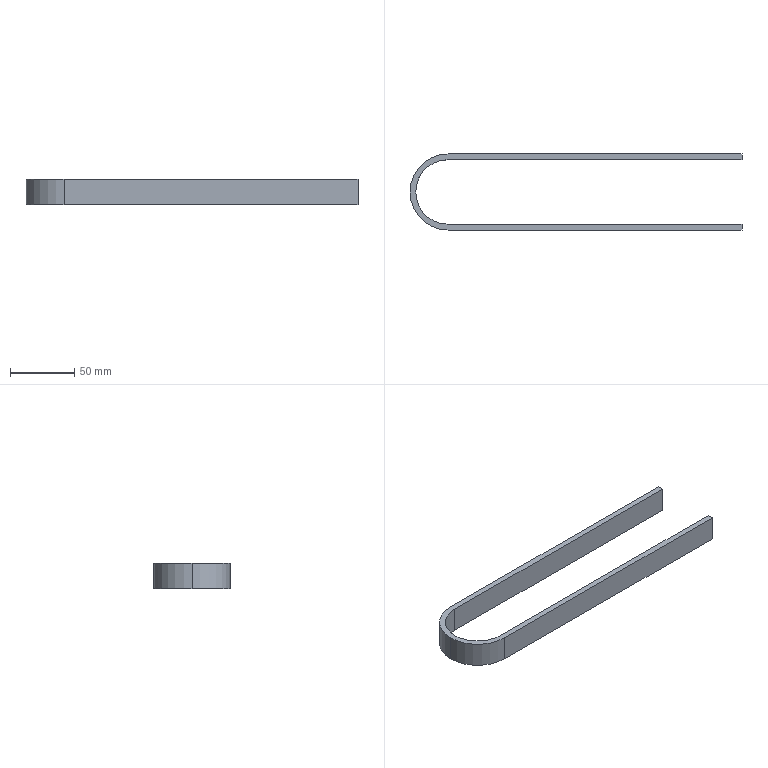Part | STEP file | Guide wheel mechanism revised.sldasm-Part-58 | 1 solid | 12 faces | box 257.5 x 59 x 20 mm | volume 48745 mm3 | plane 8 | cylinder 4 | commonest cylinder face diameters 50 x2 59 x2
STEP:
#1=CARTESIAN_POINT('',(0.,25.,10.));
#2=VERTEX_POINT('',#1);
#3=CARTESIAN_POINT('',(-25.,0.,10.));
#4=VERTEX_POINT('',#3);
#5=CARTESIAN_POINT('',(0.,0.,10.));
#6=DIRECTION('',(0.,0.,1.));
#7=DIRECTION('',(1.,0.,0.));
#8=AXIS2_PLACEMENT_3D('',#5,#6,#7);
#9=CIRCLE('',#8,25.);
#10=EDGE_CURVE('',#2,#4,#9,.T.);
#11=ORIENTED_EDGE('',*,*,#10,.T.);
#12=CARTESIAN_POINT('',(-25.,0.,-10.));
#13=VERTEX_POINT('',#12);
#14=CARTESIAN_POINT('',(-25.,0.,10.));
#15=DIRECTION('',(0.,0.,-1.));
#16=VECTOR('',#15,1000.);
#17=LINE('',#14,#16);
#18=EDGE_CURVE('',#4,#13,#17,.T.);
#19=ORIENTED_EDGE('',*,*,#18,.T.);
#20=CARTESIAN_POINT('',(0.,25.,-10.));
#21=VERTEX_POINT('',#20);
#22=CARTESIAN_POINT('',(0.,0.,-10.));
#23=DIRECTION('',(0.,0.,1.));
#24=DIRECTION('',(1.,0.,0.));
#25=AXIS2_PLACEMENT_3D('',#22,#23,#24);
#26=CIRCLE('',#25,25.);
#27=EDGE_CURVE('',#21,#13,#26,.T.);
#28=ORIENTED_EDGE('',*,*,#27,.F.);
#29=CARTESIAN_POINT('',(0.,25.,10.));
#30=DIRECTION('',(0.,0.,-1.));
#31=VECTOR('',#30,1000.);
#32=LINE('',#29,#31);
#33=EDGE_CURVE('',#2,#21,#32,.T.);
#34=ORIENTED_EDGE('',*,*,#33,.F.);
#35=EDGE_LOOP('',(#11,#19,#28,#34));
#36=FACE_OUTER_BOUND('',#35,.T.);
#37=CARTESIAN_POINT('',(0.,0.,10.));
#38=DIRECTION('',(0.,0.,-1.));
#39=DIRECTION('',(-1.,0.,0.));
#40=AXIS2_PLACEMENT_3D('',#37,#38,#39);
#41=CYLINDRICAL_SURFACE('',#40,25.);
#42=ADVANCED_FACE('',(#36),#41,.F.);
#43=CARTESIAN_POINT('',(-29.5,0.,10.));
#44=VERTEX_POINT('',#43);
#45=CARTESIAN_POINT('',(0.,-29.5,10.));
#46=VERTEX_POINT('',#45);
#47=CARTESIAN_POINT('',(0.,0.,10.));
#48=DIRECTION('',(0.,0.,1.));
#49=DIRECTION('',(1.,0.,0.));
#50=AXIS2_PLACEMENT_3D('',#47,#48,#49);
#51=CIRCLE('',#50,29.5);
#52=EDGE_CURVE('',#44,#46,#51,.T.);
#53=ORIENTED_EDGE('',*,*,#52,.F.);
#54=CARTESIAN_POINT('',(-29.5,0.,-10.));
#55=VERTEX_POINT('',#54);
#56=CARTESIAN_POINT('',(-29.5,0.,10.));
#57=DIRECTION('',(0.,0.,-1.));
#58=VECTOR('',#57,1000.);
#59=LINE('',#56,#58);
#60=EDGE_CURVE('',#44,#55,#59,.T.);
#61=ORIENTED_EDGE('',*,*,#60,.T.);
#62=CARTESIAN_POINT('',(0.,-29.5,-10.));
#63=VERTEX_POINT('',#62);
#64=CARTESIAN_POINT('',(0.,0.,-10.));
#65=DIRECTION('',(0.,0.,1.));
#66=DIRECTION('',(1.,0.,0.));
#67=AXIS2_PLACEMENT_3D('',#64,#65,#66);
#68=CIRCLE('',#67,29.5);
#69=EDGE_CURVE('',#55,#63,#68,.T.);
#70=ORIENTED_EDGE('',*,*,#69,.T.);
#71=CARTESIAN_POINT('',(0.,-29.5,10.));
#72=DIRECTION('',(0.,0.,-1.));
#73=VECTOR('',#72,1000.);
#74=LINE('',#71,#73);
#75=EDGE_CURVE('',#46,#63,#74,.T.);
#76=ORIENTED_EDGE('',*,*,#75,.F.);
#77=EDGE_LOOP('',(#53,#61,#70,#76));
#78=FACE_OUTER_BOUND('',#77,.T.);
#79=CARTESIAN_POINT('',(0.,0.,10.));
#80=DIRECTION('',(0.,0.,-1.));
#81=DIRECTION('',(-1.,0.,0.));
#82=AXIS2_PLACEMENT_3D('',#79,#80,#81);
#83=CYLINDRICAL_SURFACE('',#82,29.5);
#84=ADVANCED_FACE('',(#78),#83,.T.);
#85=CARTESIAN_POINT('',(228.,29.5,10.));
#86=VERTEX_POINT('',#85);
#87=CARTESIAN_POINT('',(228.,25.,10.));
#88=VERTEX_POINT('',#87);
#89=CARTESIAN_POINT('',(228.,0.,10.));
#90=DIRECTION('',(0.,-1.,0.));
#91=VECTOR('',#90,1000.);
#92=LINE('',#89,#91);
#93=EDGE_CURVE('',#86,#88,#92,.T.);
#94=ORIENTED_EDGE('',*,*,#93,.F.);
#95=CARTESIAN_POINT('',(0.,29.5,10.));
#96=VERTEX_POINT('',#95);
#97=CARTESIAN_POINT('',(1300.,29.5,10.));
#98=DIRECTION('',(-1.,0.,0.));
#99=VECTOR('',#98,1000.);
#100=LINE('',#97,#99);
#101=EDGE_CURVE('',#86,#96,#100,.T.);
#102=ORIENTED_EDGE('',*,*,#101,.T.);
#103=CARTESIAN_POINT('',(0.,0.,10.));
#104=DIRECTION('',(0.,0.,1.));
#105=DIRECTION('',(1.,0.,0.));
#106=AXIS2_PLACEMENT_3D('',#103,#104,#105);
#107=CIRCLE('',#106,29.5);
#108=EDGE_CURVE('',#96,#44,#107,.T.);
#109=ORIENTED_EDGE('',*,*,#108,.T.);
#110=ORIENTED_EDGE('',*,*,#52,.T.);
#111=CARTESIAN_POINT('',(228.,-29.5,10.));
#112=VERTEX_POINT('',#111);
#113=CARTESIAN_POINT('',(0.,-29.5,10.));
#114=DIRECTION('',(1.,0.,0.));
#115=VECTOR('',#114,1000.);
#116=LINE('',#113,#115);
#117=EDGE_CURVE('',#46,#112,#116,.T.);
#118=ORIENTED_EDGE('',*,*,#117,.T.);
#119=CARTESIAN_POINT('',(228.,-25.,10.));
#120=VERTEX_POINT('',#119);
#121=CARTESIAN_POINT('',(228.,0.,10.));
#122=DIRECTION('',(0.,-1.,0.));
#123=VECTOR('',#122,1000.);
#124=LINE('',#121,#123);
#125=EDGE_CURVE('',#120,#112,#124,.T.);
#126=ORIENTED_EDGE('',*,*,#125,.F.);
#127=CARTESIAN_POINT('',(0.,-25.,10.));
#128=VERTEX_POINT('',#127);
#129=CARTESIAN_POINT('',(0.,-25.,10.));
#130=DIRECTION('',(1.,0.,0.));
#131=VECTOR('',#130,1000.);
#132=LINE('',#129,#131);
#133=EDGE_CURVE('',#128,#120,#132,.T.);
#134=ORIENTED_EDGE('',*,*,#133,.F.);
#135=CARTESIAN_POINT('',(0.,0.,10.));
#136=DIRECTION('',(0.,0.,1.));
#137=DIRECTION('',(1.,0.,0.));
#138=AXIS2_PLACEMENT_3D('',#135,#136,#137);
#139=CIRCLE('',#138,25.);
#140=EDGE_CURVE('',#4,#128,#139,.T.);
#141=ORIENTED_EDGE('',*,*,#140,.F.);
#142=ORIENTED_EDGE('',*,*,#10,.F.);
#143=CARTESIAN_POINT('',(1300.,25.,10.));
#144=DIRECTION('',(-1.,0.,0.));
#145=VECTOR('',#144,1000.);
#146=LINE('',#143,#145);
#147=EDGE_CURVE('',#88,#2,#146,.T.);
#148=ORIENTED_EDGE('',*,*,#147,.F.);
#149=EDGE_LOOP('',(#94,#102,#109,#110,#118,#126,#134,#141,#142,#148));
#150=FACE_OUTER_BOUND('',#149,.T.);
#151=CARTESIAN_POINT('',(0.,0.,10.));
#152=DIRECTION('',(0.,0.,1.));
#153=DIRECTION('',(1.,0.,0.));
#154=AXIS2_PLACEMENT_3D('',#151,#152,#153);
#155=PLANE('',#154);
#156=ADVANCED_FACE('',(#150),#155,.T.);
#157=CARTESIAN_POINT('',(228.,-29.5,-10.));
#158=VERTEX_POINT('',#157);
#159=CARTESIAN_POINT('',(0.,-29.5,-10.));
#160=DIRECTION('',(1.,0.,0.));
#161=VECTOR('',#160,1000.);
#162=LINE('',#159,#161);
#163=EDGE_CURVE('',#63,#158,#162,.T.);
#164=ORIENTED_EDGE('',*,*,#163,.T.);
#165=CARTESIAN_POINT('',(228.,-29.5,10.));
#166=DIRECTION('',(0.,0.,1.));
#167=VECTOR('',#166,1000.);
#168=LINE('',#165,#167);
#169=EDGE_CURVE('',#158,#112,#168,.T.);
#170=ORIENTED_EDGE('',*,*,#169,.T.);
#171=ORIENTED_EDGE('',*,*,#117,.F.);
#172=ORIENTED_EDGE('',*,*,#75,.T.);
#173=EDGE_LOOP('',(#164,#170,#171,#172));
#174=FACE_OUTER_BOUND('',#173,.T.);
#175=CARTESIAN_POINT('',(650.,-29.5,10.));
#176=DIRECTION('',(0.,1.,0.));
#177=DIRECTION('',(-1.,0.,0.));
#178=AXIS2_PLACEMENT_3D('',#175,#176,#177);
#179=PLANE('',#178);
#180=ADVANCED_FACE('',(#174),#179,.F.);
#181=ORIENTED_EDGE('',*,*,#101,.F.);
#182=CARTESIAN_POINT('',(228.,29.5,-10.));
#183=VERTEX_POINT('',#182);
#184=CARTESIAN_POINT('',(228.,29.5,-15.));
#185=DIRECTION('',(0.,0.,1.));
#186=VECTOR('',#185,1000.);
#187=LINE('',#184,#186);
#188=EDGE_CURVE('',#183,#86,#187,.T.);
#189=ORIENTED_EDGE('',*,*,#188,.F.);
#190=CARTESIAN_POINT('',(0.,29.5,-10.));
#191=VERTEX_POINT('',#190);
#192=CARTESIAN_POINT('',(1300.,29.5,-10.));
#193=DIRECTION('',(-1.,0.,0.));
#194=VECTOR('',#193,1000.);
#195=LINE('',#192,#194);
#196=EDGE_CURVE('',#183,#191,#195,.T.);
#197=ORIENTED_EDGE('',*,*,#196,.T.);
#198=CARTESIAN_POINT('',(0.,29.5,10.));
#199=DIRECTION('',(0.,0.,-1.));
#200=VECTOR('',#199,1000.);
#201=LINE('',#198,#200);
#202=EDGE_CURVE('',#96,#191,#201,.T.);
#203=ORIENTED_EDGE('',*,*,#202,.F.);
#204=EDGE_LOOP('',(#181,#189,#197,#203));
#205=FACE_OUTER_BOUND('',#204,.T.);
#206=CARTESIAN_POINT('',(1300.,29.5,10.));
#207=DIRECTION('',(0.,-1.,0.));
#208=DIRECTION('',(0.,0.,-1.));
#209=AXIS2_PLACEMENT_3D('',#206,#207,#208);
#210=PLANE('',#209);
#211=ADVANCED_FACE('',(#205),#210,.F.);
#212=CARTESIAN_POINT('',(228.,-25.,-10.));
#213=VERTEX_POINT('',#212);
#214=CARTESIAN_POINT('',(228.,-25.,10.));
#215=DIRECTION('',(0.,0.,1.));
#216=VECTOR('',#215,1000.);
#217=LINE('',#214,#216);
#218=EDGE_CURVE('',#213,#120,#217,.T.);
#219=ORIENTED_EDGE('',*,*,#218,.F.);
#220=CARTESIAN_POINT('',(0.,-25.,-10.));
#221=VERTEX_POINT('',#220);
#222=CARTESIAN_POINT('',(0.,-25.,-10.));
#223=DIRECTION('',(1.,0.,0.));
#224=VECTOR('',#223,1000.);
#225=LINE('',#222,#224);
#226=EDGE_CURVE('',#221,#213,#225,.T.);
#227=ORIENTED_EDGE('',*,*,#226,.F.);
#228=CARTESIAN_POINT('',(0.,-25.,10.));
#229=DIRECTION('',(0.,0.,-1.));
#230=VECTOR('',#229,1000.);
#231=LINE('',#228,#230);
#232=EDGE_CURVE('',#128,#221,#231,.T.);
#233=ORIENTED_EDGE('',*,*,#232,.F.);
#234=ORIENTED_EDGE('',*,*,#133,.T.);
#235=EDGE_LOOP('',(#219,#227,#233,#234));
#236=FACE_OUTER_BOUND('',#235,.T.);
#237=CARTESIAN_POINT('',(650.,-25.,10.));
#238=DIRECTION('',(0.,1.,0.));
#239=DIRECTION('',(-1.,0.,0.));
#240=AXIS2_PLACEMENT_3D('',#237,#238,#239);
#241=PLANE('',#240);
#242=ADVANCED_FACE('',(#236),#241,.T.);
#243=CARTESIAN_POINT('',(228.,25.,-10.));
#244=VERTEX_POINT('',#243);
#245=CARTESIAN_POINT('',(228.,25.,10.));
#246=DIRECTION('',(0.,0.,-1.));
#247=VECTOR('',#246,1000.);
#248=LINE('',#245,#247);
#249=EDGE_CURVE('',#88,#244,#248,.T.);
#250=ORIENTED_EDGE('',*,*,#249,.F.);
#251=ORIENTED_EDGE('',*,*,#147,.T.);
#252=ORIENTED_EDGE('',*,*,#33,.T.);
#253=CARTESIAN_POINT('',(1300.,25.,-10.));
#254=DIRECTION('',(-1.,0.,0.));
#255=VECTOR('',#254,1000.);
#256=LINE('',#253,#255);
#257=EDGE_CURVE('',#244,#21,#256,.T.);
#258=ORIENTED_EDGE('',*,*,#257,.F.);
#259=EDGE_LOOP('',(#250,#251,#252,#258));
#260=FACE_OUTER_BOUND('',#259,.T.);
#261=CARTESIAN_POINT('',(1300.,25.,10.));
#262=DIRECTION('',(0.,-1.,0.));
#263=DIRECTION('',(0.,0.,-1.));
#264=AXIS2_PLACEMENT_3D('',#261,#262,#263);
#265=PLANE('',#264);
#266=ADVANCED_FACE('',(#260),#265,.T.);
#267=ORIENTED_EDGE('',*,*,#196,.F.);
#268=CARTESIAN_POINT('',(228.,0.,-10.));
#269=DIRECTION('',(0.,-1.,0.));
#270=VECTOR('',#269,1000.);
#271=LINE('',#268,#270);
#272=EDGE_CURVE('',#183,#244,#271,.T.);
#273=ORIENTED_EDGE('',*,*,#272,.T.);
#274=ORIENTED_EDGE('',*,*,#257,.T.);
#275=ORIENTED_EDGE('',*,*,#27,.T.);
#276=CARTESIAN_POINT('',(0.,0.,-10.));
#277=DIRECTION('',(0.,0.,1.));
#278=DIRECTION('',(1.,0.,0.));
#279=AXIS2_PLACEMENT_3D('',#276,#277,#278);
#280=CIRCLE('',#279,25.);
#281=EDGE_CURVE('',#13,#221,#280,.T.);
#282=ORIENTED_EDGE('',*,*,#281,.T.);
#283=ORIENTED_EDGE('',*,*,#226,.T.);
#284=CARTESIAN_POINT('',(228.,0.,-10.));
#285=DIRECTION('',(0.,-1.,0.));
#286=VECTOR('',#285,1000.);
#287=LINE('',#284,#286);
#288=EDGE_CURVE('',#213,#158,#287,.T.);
#289=ORIENTED_EDGE('',*,*,#288,.T.);
#290=ORIENTED_EDGE('',*,*,#163,.F.);
#291=ORIENTED_EDGE('',*,*,#69,.F.);
#292=CARTESIAN_POINT('',(0.,0.,-10.));
#293=DIRECTION('',(0.,0.,1.));
#294=DIRECTION('',(1.,0.,0.));
#295=AXIS2_PLACEMENT_3D('',#292,#293,#294);
#296=CIRCLE('',#295,29.5);
#297=EDGE_CURVE('',#191,#55,#296,.T.);
#298=ORIENTED_EDGE('',*,*,#297,.F.);
#299=EDGE_LOOP('',(#267,#273,#274,#275,#282,#283,#289,#290,#291,#298));
#300=FACE_OUTER_BOUND('',#299,.T.);
#301=CARTESIAN_POINT('',(0.,0.,-10.));
#302=DIRECTION('',(0.,0.,1.));
#303=DIRECTION('',(1.,0.,0.));
#304=AXIS2_PLACEMENT_3D('',#301,#302,#303);
#305=PLANE('',#304);
#306=ADVANCED_FACE('',(#300),#305,.F.);
#307=ORIENTED_EDGE('',*,*,#60,.F.);
#308=ORIENTED_EDGE('',*,*,#108,.F.);
#309=ORIENTED_EDGE('',*,*,#202,.T.);
#310=ORIENTED_EDGE('',*,*,#297,.T.);
#311=EDGE_LOOP('',(#307,#308,#309,#310));
#312=FACE_OUTER_BOUND('',#311,.T.);
#313=CARTESIAN_POINT('',(0.,0.,10.));
#314=DIRECTION('',(0.,0.,-1.));
#315=DIRECTION('',(-1.,0.,0.));
#316=AXIS2_PLACEMENT_3D('',#313,#314,#315);
#317=CYLINDRICAL_SURFACE('',#316,29.5);
#318=ADVANCED_FACE('',(#312),#317,.T.);
#319=ORIENTED_EDGE('',*,*,#18,.F.);
#320=ORIENTED_EDGE('',*,*,#140,.T.);
#321=ORIENTED_EDGE('',*,*,#232,.T.);
#322=ORIENTED_EDGE('',*,*,#281,.F.);
#323=EDGE_LOOP('',(#319,#320,#321,#322));
#324=FACE_OUTER_BOUND('',#323,.T.);
#325=CARTESIAN_POINT('',(0.,0.,10.));
#326=DIRECTION('',(0.,0.,-1.));
#327=DIRECTION('',(-1.,0.,0.));
#328=AXIS2_PLACEMENT_3D('',#325,#326,#327);
#329=CYLINDRICAL_SURFACE('',#328,25.);
#330=ADVANCED_FACE('',(#324),#329,.F.);
#331=ORIENTED_EDGE('',*,*,#125,.T.);
#332=ORIENTED_EDGE('',*,*,#169,.F.);
#333=ORIENTED_EDGE('',*,*,#288,.F.);
#334=ORIENTED_EDGE('',*,*,#218,.T.);
#335=EDGE_LOOP('',(#331,#332,#333,#334));
#336=FACE_OUTER_BOUND('',#335,.T.);
#337=CARTESIAN_POINT('',(228.,-30.5,-15.));
#338=DIRECTION('',(-1.,0.,0.));
#339=DIRECTION('',(0.,0.,1.));
#340=AXIS2_PLACEMENT_3D('',#337,#338,#339);
#341=PLANE('',#340);
#342=ADVANCED_FACE('',(#336),#341,.F.);
#343=ORIENTED_EDGE('',*,*,#93,.T.);
#344=ORIENTED_EDGE('',*,*,#249,.T.);
#345=ORIENTED_EDGE('',*,*,#272,.F.);
#346=ORIENTED_EDGE('',*,*,#188,.T.);
#347=EDGE_LOOP('',(#343,#344,#345,#346));
#348=FACE_OUTER_BOUND('',#347,.T.);
#349=CARTESIAN_POINT('',(228.,-30.5,-15.));
#350=DIRECTION('',(-1.,0.,0.));
#351=DIRECTION('',(0.,0.,1.));
#352=AXIS2_PLACEMENT_3D('',#349,#350,#351);
#353=PLANE('',#352);
#354=ADVANCED_FACE('',(#348),#353,.F.);
#355=CLOSED_SHELL('',(#42,#84,#156,#180,#211,#242,#266,#306,#318,#330,#342,#354));
#356=MANIFOLD_SOLID_BREP('',#355);
#357=CARTESIAN_POINT('',(0.,0.,0.));
#358=DIRECTION('',(0.,0.,1.));
#359=DIRECTION('',(1.,0.,0.));
#360=AXIS2_PLACEMENT_3D('',#357,#358,#359);
#361=(LENGTH_UNIT()NAMED_UNIT(*)SI_UNIT(.MILLI.,.METRE.));
#362=UNCERTAINTY_MEASURE_WITH_UNIT(LENGTH_MEASURE(0.00001),#361,'','');
#363=(NAMED_UNIT(*)PLANE_ANGLE_UNIT()SI_UNIT($,.RADIAN.));
#364=(NAMED_UNIT(*)SI_UNIT($,.STERADIAN.)SOLID_ANGLE_UNIT());
#365=(GEOMETRIC_REPRESENTATION_CONTEXT(3)GLOBAL_UNCERTAINTY_ASSIGNED_CONTEXT((#362))GLOBAL_UNIT_ASSIGNED_CONTEXT((#361,#363,#364))REPRESENTATION_CONTEXT('',''));
#366=ADVANCED_BREP_SHAPE_REPRESENTATION('',(#356,#360),#365);